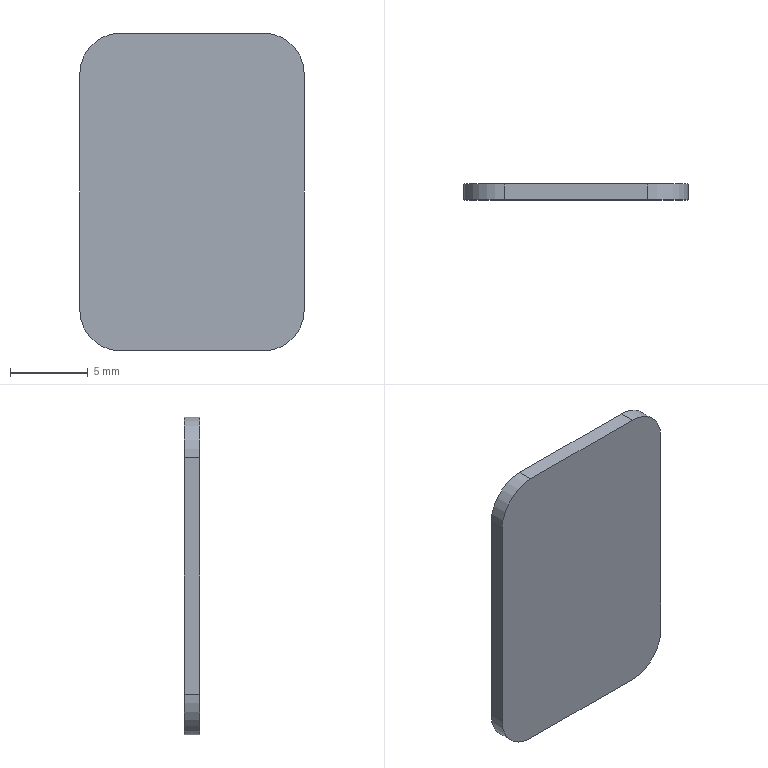Part | SolidWorks | features BaseBody 1 | 1 solid | 58 faces | box 14.4 x 1 x 20.4 mm | volume 279.954 mm3 | plane 38 | cylinder 12 | cone 8 | commonest cylinder face diameters 3.8 x8 5.2 x4